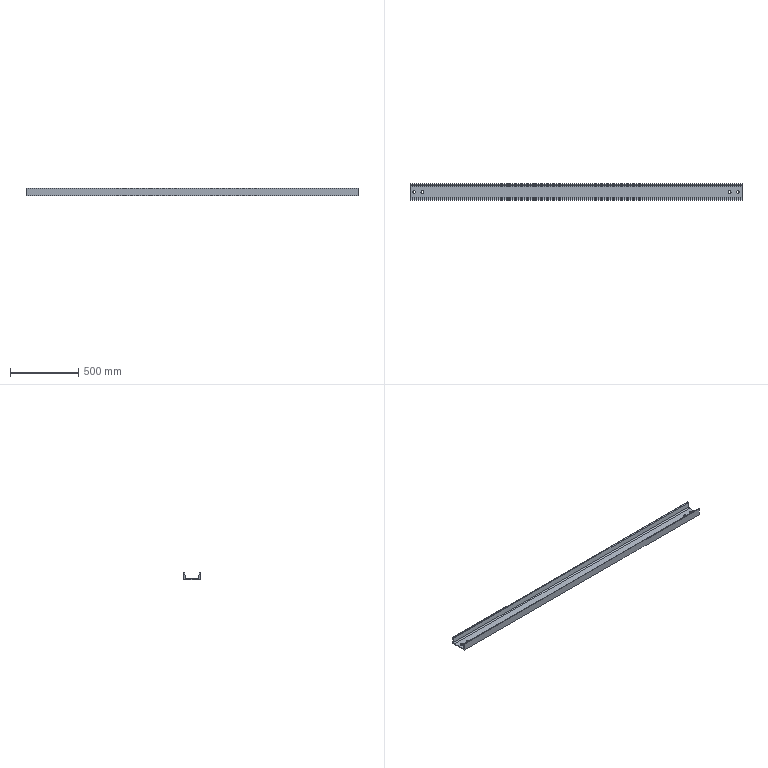Part | STEP file | E3-中转釜连接梁4_Default<As Machined> | 1 solid | 22 faces | box 2430 x 120 x 53 mm | volume 3724626 mm3 | cylinder 12 | plane 10 | commonest cylinder face diameters 19 x8 9 x2 18 x2